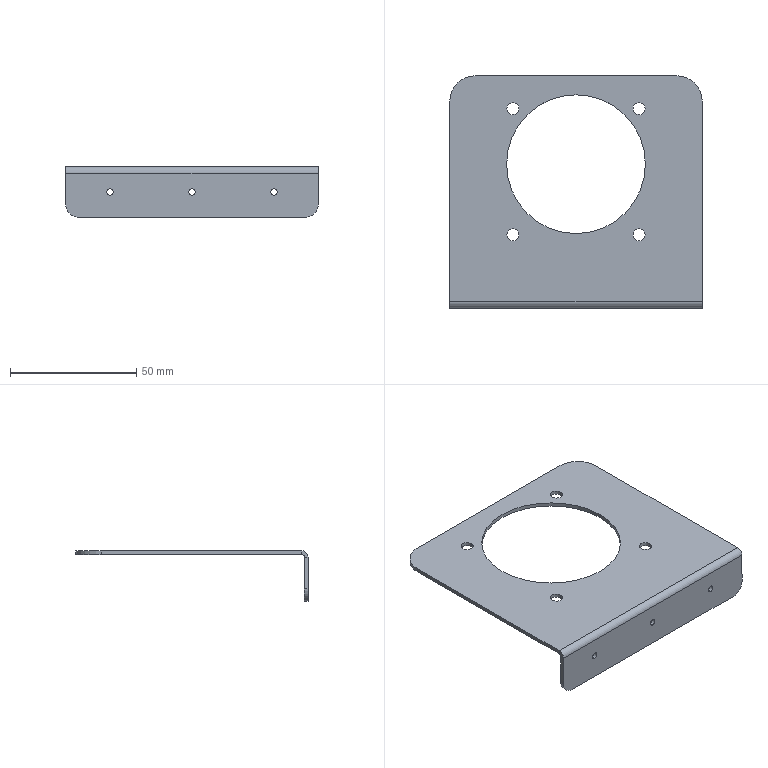Part | SolidWorks | features Fillet 2, HoleWzd 2, Cut 1, EdgeFlange 1, FlatPattern 1, ICE 1, SMBaseFlange 1, SheetMetal 1 | 1 solid | 34 faces | box 100 x 92 x 20 mm | volume 12687 mm3 | cylinder 22 | plane 12 | commonest cylinder face diameters 4.8 x8 2.5 x6 10 x2 20 x2 55 x2 2 x1
STEP:
#1=CARTESIAN_POINT('',(-32.5,-46.,-11.25));
#2=VERTEX_POINT('',#1);
#3=CARTESIAN_POINT('',(-32.5,-46.,-8.75));
#4=VERTEX_POINT('',#3);
#5=CARTESIAN_POINT('',(-32.5,-46.,-10.));
#6=DIRECTION('',(0.,1.,0.));
#7=DIRECTION('',(0.,0.,1.));
#8=AXIS2_PLACEMENT_3D('',#5,#6,#7);
#9=CIRCLE('',#8,1.25);
#10=EDGE_CURVE('',#2,#4,#9,.T.);
#11=ORIENTED_EDGE('',*,*,#10,.F.);
#12=CARTESIAN_POINT('',(-32.5,-44.5,-11.25));
#13=VERTEX_POINT('',#12);
#14=CARTESIAN_POINT('',(-32.5,-44.5,-11.25));
#15=DIRECTION('',(0.,1.,0.));
#16=VECTOR('',#15,1000.);
#17=LINE('',#14,#16);
#18=EDGE_CURVE('',#2,#13,#17,.T.);
#19=ORIENTED_EDGE('',*,*,#18,.T.);
#20=CARTESIAN_POINT('',(-32.5,-44.5,-8.75));
#21=VERTEX_POINT('',#20);
#22=CARTESIAN_POINT('',(-32.5,-44.5,-10.));
#23=DIRECTION('',(0.,1.,0.));
#24=DIRECTION('',(0.,0.,1.));
#25=AXIS2_PLACEMENT_3D('',#22,#23,#24);
#26=CIRCLE('',#25,1.25);
#27=EDGE_CURVE('',#13,#21,#26,.T.);
#28=ORIENTED_EDGE('',*,*,#27,.T.);
#29=CARTESIAN_POINT('',(-32.5,-44.5,-8.75));
#30=DIRECTION('',(0.,1.,0.));
#31=VECTOR('',#30,1000.);
#32=LINE('',#29,#31);
#33=EDGE_CURVE('',#4,#21,#32,.T.);
#34=ORIENTED_EDGE('',*,*,#33,.F.);
#35=EDGE_LOOP('',(#11,#19,#28,#34));
#36=FACE_OUTER_BOUND('',#35,.T.);
#37=CARTESIAN_POINT('',(-32.5,-44.5,-10.));
#38=DIRECTION('',(0.,1.,0.));
#39=DIRECTION('',(0.,0.,1.));
#40=AXIS2_PLACEMENT_3D('',#37,#38,#39);
#41=CYLINDRICAL_SURFACE('',#40,1.25);
#42=ADVANCED_FACE('',(#36),#41,.F.);
#43=CARTESIAN_POINT('',(0.,-46.,-11.25));
#44=VERTEX_POINT('',#43);
#45=CARTESIAN_POINT('',(0.,-46.,-8.75));
#46=VERTEX_POINT('',#45);
#47=CARTESIAN_POINT('',(0.,-46.,-10.));
#48=DIRECTION('',(0.,1.,0.));
#49=DIRECTION('',(0.,0.,1.));
#50=AXIS2_PLACEMENT_3D('',#47,#48,#49);
#51=CIRCLE('',#50,1.25);
#52=EDGE_CURVE('',#44,#46,#51,.T.);
#53=ORIENTED_EDGE('',*,*,#52,.F.);
#54=CARTESIAN_POINT('',(0.,-44.5,-11.25));
#55=VERTEX_POINT('',#54);
#56=CARTESIAN_POINT('',(0.,-44.5,-11.25));
#57=DIRECTION('',(0.,1.,0.));
#58=VECTOR('',#57,1000.);
#59=LINE('',#56,#58);
#60=EDGE_CURVE('',#44,#55,#59,.T.);
#61=ORIENTED_EDGE('',*,*,#60,.T.);
#62=CARTESIAN_POINT('',(0.,-44.5,-8.75));
#63=VERTEX_POINT('',#62);
#64=CARTESIAN_POINT('',(0.,-44.5,-10.));
#65=DIRECTION('',(0.,1.,0.));
#66=DIRECTION('',(0.,0.,1.));
#67=AXIS2_PLACEMENT_3D('',#64,#65,#66);
#68=CIRCLE('',#67,1.25);
#69=EDGE_CURVE('',#55,#63,#68,.T.);
#70=ORIENTED_EDGE('',*,*,#69,.T.);
#71=CARTESIAN_POINT('',(0.,-44.5,-8.75));
#72=DIRECTION('',(0.,1.,0.));
#73=VECTOR('',#72,1000.);
#74=LINE('',#71,#73);
#75=EDGE_CURVE('',#46,#63,#74,.T.);
#76=ORIENTED_EDGE('',*,*,#75,.F.);
#77=EDGE_LOOP('',(#53,#61,#70,#76));
#78=FACE_OUTER_BOUND('',#77,.T.);
#79=CARTESIAN_POINT('',(0.,-44.5,-10.));
#80=DIRECTION('',(0.,1.,0.));
#81=DIRECTION('',(0.,0.,1.));
#82=AXIS2_PLACEMENT_3D('',#79,#80,#81);
#83=CYLINDRICAL_SURFACE('',#82,1.25);
#84=ADVANCED_FACE('',(#78),#83,.F.);
#85=CARTESIAN_POINT('',(32.5,-46.,-11.25));
#86=VERTEX_POINT('',#85);
#87=CARTESIAN_POINT('',(32.5,-46.,-8.75));
#88=VERTEX_POINT('',#87);
#89=CARTESIAN_POINT('',(32.5,-46.,-10.));
#90=DIRECTION('',(0.,1.,0.));
#91=DIRECTION('',(0.,0.,1.));
#92=AXIS2_PLACEMENT_3D('',#89,#90,#91);
#93=CIRCLE('',#92,1.25);
#94=EDGE_CURVE('',#86,#88,#93,.T.);
#95=ORIENTED_EDGE('',*,*,#94,.F.);
#96=CARTESIAN_POINT('',(32.5,-44.5,-11.25));
#97=VERTEX_POINT('',#96);
#98=CARTESIAN_POINT('',(32.5,-44.5,-11.25));
#99=DIRECTION('',(0.,1.,0.));
#100=VECTOR('',#99,1000.);
#101=LINE('',#98,#100);
#102=EDGE_CURVE('',#86,#97,#101,.T.);
#103=ORIENTED_EDGE('',*,*,#102,.T.);
#104=CARTESIAN_POINT('',(32.5,-44.5,-8.75));
#105=VERTEX_POINT('',#104);
#106=CARTESIAN_POINT('',(32.5,-44.5,-10.));
#107=DIRECTION('',(0.,1.,0.));
#108=DIRECTION('',(0.,0.,1.));
#109=AXIS2_PLACEMENT_3D('',#106,#107,#108);
#110=CIRCLE('',#109,1.25);
#111=EDGE_CURVE('',#97,#105,#110,.T.);
#112=ORIENTED_EDGE('',*,*,#111,.T.);
#113=CARTESIAN_POINT('',(32.5,-44.5,-8.75));
#114=DIRECTION('',(0.,1.,0.));
#115=VECTOR('',#114,1000.);
#116=LINE('',#113,#115);
#117=EDGE_CURVE('',#88,#105,#116,.T.);
#118=ORIENTED_EDGE('',*,*,#117,.F.);
#119=EDGE_LOOP('',(#95,#103,#112,#118));
#120=FACE_OUTER_BOUND('',#119,.T.);
#121=CARTESIAN_POINT('',(32.5,-44.5,-10.));
#122=DIRECTION('',(0.,1.,0.));
#123=DIRECTION('',(0.,0.,1.));
#124=AXIS2_PLACEMENT_3D('',#121,#122,#123);
#125=CYLINDRICAL_SURFACE('',#124,1.25);
#126=ADVANCED_FACE('',(#120),#125,.F.);
#127=CARTESIAN_POINT('',(27.4,33.,0.));
#128=VERTEX_POINT('',#127);
#129=CARTESIAN_POINT('',(22.6,33.,0.));
#130=VERTEX_POINT('',#129);
#131=CARTESIAN_POINT('',(25.,33.,0.));
#132=DIRECTION('',(0.,0.,-1.));
#133=DIRECTION('',(-1.,0.,0.));
#134=AXIS2_PLACEMENT_3D('',#131,#132,#133);
#135=CIRCLE('',#134,2.4);
#136=EDGE_CURVE('',#128,#130,#135,.T.);
#137=ORIENTED_EDGE('',*,*,#136,.F.);
#138=CARTESIAN_POINT('',(27.4,33.,-1.5));
#139=VERTEX_POINT('',#138);
#140=CARTESIAN_POINT('',(27.4,33.,-1.5));
#141=DIRECTION('',(0.,0.,-1.));
#142=VECTOR('',#141,1000.);
#143=LINE('',#140,#142);
#144=EDGE_CURVE('',#128,#139,#143,.T.);
#145=ORIENTED_EDGE('',*,*,#144,.T.);
#146=CARTESIAN_POINT('',(22.6,33.,-1.5));
#147=VERTEX_POINT('',#146);
#148=CARTESIAN_POINT('',(25.,33.,-1.5));
#149=DIRECTION('',(0.,0.,-1.));
#150=DIRECTION('',(-1.,0.,0.));
#151=AXIS2_PLACEMENT_3D('',#148,#149,#150);
#152=CIRCLE('',#151,2.4);
#153=EDGE_CURVE('',#139,#147,#152,.T.);
#154=ORIENTED_EDGE('',*,*,#153,.T.);
#155=CARTESIAN_POINT('',(22.6,33.,-1.5));
#156=DIRECTION('',(0.,0.,-1.));
#157=VECTOR('',#156,1000.);
#158=LINE('',#155,#157);
#159=EDGE_CURVE('',#130,#147,#158,.T.);
#160=ORIENTED_EDGE('',*,*,#159,.F.);
#161=EDGE_LOOP('',(#137,#145,#154,#160));
#162=FACE_OUTER_BOUND('',#161,.T.);
#163=CARTESIAN_POINT('',(25.,33.,-1.5));
#164=DIRECTION('',(0.,0.,-1.));
#165=DIRECTION('',(-1.,0.,0.));
#166=AXIS2_PLACEMENT_3D('',#163,#164,#165);
#167=CYLINDRICAL_SURFACE('',#166,2.4);
#168=ADVANCED_FACE('',(#162),#167,.F.);
#169=CARTESIAN_POINT('',(27.4,-17.,0.));
#170=VERTEX_POINT('',#169);
#171=CARTESIAN_POINT('',(22.6,-17.,0.));
#172=VERTEX_POINT('',#171);
#173=CARTESIAN_POINT('',(25.,-17.,0.));
#174=DIRECTION('',(0.,0.,-1.));
#175=DIRECTION('',(-1.,0.,0.));
#176=AXIS2_PLACEMENT_3D('',#173,#174,#175);
#177=CIRCLE('',#176,2.4);
#178=EDGE_CURVE('',#170,#172,#177,.T.);
#179=ORIENTED_EDGE('',*,*,#178,.F.);
#180=CARTESIAN_POINT('',(27.4,-17.,-1.5));
#181=VERTEX_POINT('',#180);
#182=CARTESIAN_POINT('',(27.4,-17.,-1.5));
#183=DIRECTION('',(0.,0.,-1.));
#184=VECTOR('',#183,1000.);
#185=LINE('',#182,#184);
#186=EDGE_CURVE('',#170,#181,#185,.T.);
#187=ORIENTED_EDGE('',*,*,#186,.T.);
#188=CARTESIAN_POINT('',(22.6,-17.,-1.5));
#189=VERTEX_POINT('',#188);
#190=CARTESIAN_POINT('',(25.,-17.,-1.5));
#191=DIRECTION('',(0.,0.,-1.));
#192=DIRECTION('',(-1.,0.,0.));
#193=AXIS2_PLACEMENT_3D('',#190,#191,#192);
#194=CIRCLE('',#193,2.4);
#195=EDGE_CURVE('',#181,#189,#194,.T.);
#196=ORIENTED_EDGE('',*,*,#195,.T.);
#197=CARTESIAN_POINT('',(22.6,-17.,-1.5));
#198=DIRECTION('',(0.,0.,-1.));
#199=VECTOR('',#198,1000.);
#200=LINE('',#197,#199);
#201=EDGE_CURVE('',#172,#189,#200,.T.);
#202=ORIENTED_EDGE('',*,*,#201,.F.);
#203=EDGE_LOOP('',(#179,#187,#196,#202));
#204=FACE_OUTER_BOUND('',#203,.T.);
#205=CARTESIAN_POINT('',(25.,-17.,-1.5));
#206=DIRECTION('',(0.,0.,-1.));
#207=DIRECTION('',(-1.,0.,0.));
#208=AXIS2_PLACEMENT_3D('',#205,#206,#207);
#209=CYLINDRICAL_SURFACE('',#208,2.4);
#210=ADVANCED_FACE('',(#204),#209,.F.);
#211=CARTESIAN_POINT('',(-22.6,-17.,0.));
#212=VERTEX_POINT('',#211);
#213=CARTESIAN_POINT('',(-27.4,-17.,0.));
#214=VERTEX_POINT('',#213);
#215=CARTESIAN_POINT('',(-25.,-17.,0.));
#216=DIRECTION('',(0.,0.,-1.));
#217=DIRECTION('',(-1.,0.,0.));
#218=AXIS2_PLACEMENT_3D('',#215,#216,#217);
#219=CIRCLE('',#218,2.4);
#220=EDGE_CURVE('',#212,#214,#219,.T.);
#221=ORIENTED_EDGE('',*,*,#220,.F.);
#222=CARTESIAN_POINT('',(-22.6,-17.,-1.5));
#223=VERTEX_POINT('',#222);
#224=CARTESIAN_POINT('',(-22.6,-17.,-1.5));
#225=DIRECTION('',(0.,0.,-1.));
#226=VECTOR('',#225,1000.);
#227=LINE('',#224,#226);
#228=EDGE_CURVE('',#212,#223,#227,.T.);
#229=ORIENTED_EDGE('',*,*,#228,.T.);
#230=CARTESIAN_POINT('',(-27.4,-17.,-1.5));
#231=VERTEX_POINT('',#230);
#232=CARTESIAN_POINT('',(-25.,-17.,-1.5));
#233=DIRECTION('',(0.,0.,-1.));
#234=DIRECTION('',(-1.,0.,0.));
#235=AXIS2_PLACEMENT_3D('',#232,#233,#234);
#236=CIRCLE('',#235,2.4);
#237=EDGE_CURVE('',#223,#231,#236,.T.);
#238=ORIENTED_EDGE('',*,*,#237,.T.);
#239=CARTESIAN_POINT('',(-27.4,-17.,-1.5));
#240=DIRECTION('',(0.,0.,-1.));
#241=VECTOR('',#240,1000.);
#242=LINE('',#239,#241);
#243=EDGE_CURVE('',#214,#231,#242,.T.);
#244=ORIENTED_EDGE('',*,*,#243,.F.);
#245=EDGE_LOOP('',(#221,#229,#238,#244));
#246=FACE_OUTER_BOUND('',#245,.T.);
#247=CARTESIAN_POINT('',(-25.,-17.,-1.5));
#248=DIRECTION('',(0.,0.,-1.));
#249=DIRECTION('',(-1.,0.,0.));
#250=AXIS2_PLACEMENT_3D('',#247,#248,#249);
#251=CYLINDRICAL_SURFACE('',#250,2.4);
#252=ADVANCED_FACE('',(#246),#251,.F.);
#253=CARTESIAN_POINT('',(-22.6,33.,0.));
#254=VERTEX_POINT('',#253);
#255=CARTESIAN_POINT('',(-27.4,33.,0.));
#256=VERTEX_POINT('',#255);
#257=CARTESIAN_POINT('',(-25.,33.,0.));
#258=DIRECTION('',(0.,0.,-1.));
#259=DIRECTION('',(-1.,0.,0.));
#260=AXIS2_PLACEMENT_3D('',#257,#258,#259);
#261=CIRCLE('',#260,2.4);
#262=EDGE_CURVE('',#254,#256,#261,.T.);
#263=ORIENTED_EDGE('',*,*,#262,.F.);
#264=CARTESIAN_POINT('',(-22.6,33.,-1.5));
#265=VERTEX_POINT('',#264);
#266=CARTESIAN_POINT('',(-22.6,33.,-1.5));
#267=DIRECTION('',(0.,0.,-1.));
#268=VECTOR('',#267,1000.);
#269=LINE('',#266,#268);
#270=EDGE_CURVE('',#254,#265,#269,.T.);
#271=ORIENTED_EDGE('',*,*,#270,.T.);
#272=CARTESIAN_POINT('',(-27.4,33.,-1.5));
#273=VERTEX_POINT('',#272);
#274=CARTESIAN_POINT('',(-25.,33.,-1.5));
#275=DIRECTION('',(0.,0.,-1.));
#276=DIRECTION('',(-1.,0.,0.));
#277=AXIS2_PLACEMENT_3D('',#274,#275,#276);
#278=CIRCLE('',#277,2.4);
#279=EDGE_CURVE('',#265,#273,#278,.T.);
#280=ORIENTED_EDGE('',*,*,#279,.T.);
#281=CARTESIAN_POINT('',(-27.4,33.,-1.5));
#282=DIRECTION('',(0.,0.,-1.));
#283=VECTOR('',#282,1000.);
#284=LINE('',#281,#283);
#285=EDGE_CURVE('',#256,#273,#284,.T.);
#286=ORIENTED_EDGE('',*,*,#285,.F.);
#287=EDGE_LOOP('',(#263,#271,#280,#286));
#288=FACE_OUTER_BOUND('',#287,.T.);
#289=CARTESIAN_POINT('',(-25.,33.,-1.5));
#290=DIRECTION('',(0.,0.,-1.));
#291=DIRECTION('',(-1.,0.,0.));
#292=AXIS2_PLACEMENT_3D('',#289,#290,#291);
#293=CYLINDRICAL_SURFACE('',#292,2.4);
#294=ADVANCED_FACE('',(#288),#293,.F.);
#295=CARTESIAN_POINT('',(-27.5,11.,0.));
#296=VERTEX_POINT('',#295);
#297=CARTESIAN_POINT('',(27.5,11.,0.));
#298=VERTEX_POINT('',#297);
#299=CARTESIAN_POINT('',(0.,11.,0.));
#300=DIRECTION('',(0.,0.,1.));
#301=DIRECTION('',(1.,0.,0.));
#302=AXIS2_PLACEMENT_3D('',#299,#300,#301);
#303=CIRCLE('',#302,27.5);
#304=EDGE_CURVE('',#296,#298,#303,.T.);
#305=ORIENTED_EDGE('',*,*,#304,.T.);
#306=CARTESIAN_POINT('',(27.5,11.,-1.5));
#307=VERTEX_POINT('',#306);
#308=CARTESIAN_POINT('',(27.5,11.,8.5));
#309=DIRECTION('',(0.,0.,-1.));
#310=VECTOR('',#309,1000.);
#311=LINE('',#308,#310);
#312=EDGE_CURVE('',#298,#307,#311,.T.);
#313=ORIENTED_EDGE('',*,*,#312,.T.);
#314=CARTESIAN_POINT('',(-27.5,11.,-1.5));
#315=VERTEX_POINT('',#314);
#316=CARTESIAN_POINT('',(0.,11.,-1.5));
#317=DIRECTION('',(0.,0.,-1.));
#318=DIRECTION('',(-1.,0.,0.));
#319=AXIS2_PLACEMENT_3D('',#316,#317,#318);
#320=CIRCLE('',#319,27.5);
#321=EDGE_CURVE('',#307,#315,#320,.T.);
#322=ORIENTED_EDGE('',*,*,#321,.T.);
#323=CARTESIAN_POINT('',(-27.5,11.,8.5));
#324=DIRECTION('',(0.,0.,-1.));
#325=VECTOR('',#324,1000.);
#326=LINE('',#323,#325);
#327=EDGE_CURVE('',#296,#315,#326,.T.);
#328=ORIENTED_EDGE('',*,*,#327,.F.);
#329=EDGE_LOOP('',(#305,#313,#322,#328));
#330=FACE_OUTER_BOUND('',#329,.T.);
#331=CARTESIAN_POINT('',(0.,11.,8.5));
#332=DIRECTION('',(0.,0.,-1.));
#333=DIRECTION('',(-1.,0.,0.));
#334=AXIS2_PLACEMENT_3D('',#331,#332,#333);
#335=CYLINDRICAL_SURFACE('',#334,27.5);
#336=ADVANCED_FACE('',(#330),#335,.F.);
#337=CARTESIAN_POINT('',(0.,-44.5,-10.));
#338=DIRECTION('',(0.,1.,0.));
#339=DIRECTION('',(0.,0.,1.));
#340=AXIS2_PLACEMENT_3D('',#337,#338,#339);
#341=CIRCLE('',#340,1.25);
#342=EDGE_CURVE('',#63,#55,#341,.T.);
#343=ORIENTED_EDGE('',*,*,#342,.F.);
#344=ORIENTED_EDGE('',*,*,#69,.F.);
#345=EDGE_LOOP('',(#343,#344));
#346=FACE_BOUND('',#345,.T.);
#347=CARTESIAN_POINT('',(50.,-44.5,-2.5));
#348=VERTEX_POINT('',#347);
#349=CARTESIAN_POINT('',(50.,-44.5,-15.));
#350=VERTEX_POINT('',#349);
#351=CARTESIAN_POINT('',(50.,-44.5,0.));
#352=DIRECTION('',(0.,0.,-1.));
#353=VECTOR('',#352,1000.);
#354=LINE('',#351,#353);
#355=EDGE_CURVE('',#348,#350,#354,.T.);
#356=ORIENTED_EDGE('',*,*,#355,.T.);
#357=CARTESIAN_POINT('',(45.,-44.5,-20.));
#358=VERTEX_POINT('',#357);
#359=CARTESIAN_POINT('',(45.,-44.5,-15.));
#360=DIRECTION('',(0.,1.,0.));
#361=DIRECTION('',(0.,0.,-1.));
#362=AXIS2_PLACEMENT_3D('',#359,#360,#361);
#363=CIRCLE('',#362,5.);
#364=EDGE_CURVE('',#350,#358,#363,.T.);
#365=ORIENTED_EDGE('',*,*,#364,.T.);
#366=CARTESIAN_POINT('',(-45.,-44.5,-20.));
#367=VERTEX_POINT('',#366);
#368=CARTESIAN_POINT('',(0.,-44.5,-20.));
#369=DIRECTION('',(-1.,0.,0.));
#370=VECTOR('',#369,1000.);
#371=LINE('',#368,#370);
#372=EDGE_CURVE('',#358,#367,#371,.T.);
#373=ORIENTED_EDGE('',*,*,#372,.T.);
#374=CARTESIAN_POINT('',(-50.,-44.5,-15.));
#375=VERTEX_POINT('',#374);
#376=CARTESIAN_POINT('',(-45.,-44.5,-15.));
#377=DIRECTION('',(0.,1.,0.));
#378=DIRECTION('',(0.,0.,-1.));
#379=AXIS2_PLACEMENT_3D('',#376,#377,#378);
#380=CIRCLE('',#379,5.);
#381=EDGE_CURVE('',#367,#375,#380,.T.);
#382=ORIENTED_EDGE('',*,*,#381,.T.);
#383=CARTESIAN_POINT('',(-50.,-44.5,-2.5));
#384=VERTEX_POINT('',#383);
#385=CARTESIAN_POINT('',(-50.,-44.5,0.));
#386=DIRECTION('',(0.,0.,1.));
#387=VECTOR('',#386,1000.);
#388=LINE('',#385,#387);
#389=EDGE_CURVE('',#375,#384,#388,.T.);
#390=ORIENTED_EDGE('',*,*,#389,.T.);
#391=CARTESIAN_POINT('',(50.,-44.5,-2.5));
#392=DIRECTION('',(-1.,0.,0.));
#393=VECTOR('',#392,1000.);
#394=LINE('',#391,#393);
#395=EDGE_CURVE('',#348,#384,#394,.T.);
#396=ORIENTED_EDGE('',*,*,#395,.F.);
#397=EDGE_LOOP('',(#356,#365,#373,#382,#390,#396));
#398=FACE_OUTER_BOUND('',#397,.T.);
#399=CARTESIAN_POINT('',(32.5,-44.5,-10.));
#400=DIRECTION('',(0.,1.,0.));
#401=DIRECTION('',(0.,0.,1.));
#402=AXIS2_PLACEMENT_3D('',#399,#400,#401);
#403=CIRCLE('',#402,1.25);
#404=EDGE_CURVE('',#105,#97,#403,.T.);
#405=ORIENTED_EDGE('',*,*,#404,.F.);
#406=ORIENTED_EDGE('',*,*,#111,.F.);
#407=EDGE_LOOP('',(#405,#406));
#408=FACE_BOUND('',#407,.T.);
#409=CARTESIAN_POINT('',(-32.5,-44.5,-10.));
#410=DIRECTION('',(0.,1.,0.));
#411=DIRECTION('',(0.,0.,1.));
#412=AXIS2_PLACEMENT_3D('',#409,#410,#411);
#413=CIRCLE('',#412,1.25);
#414=EDGE_CURVE('',#21,#13,#413,.T.);
#415=ORIENTED_EDGE('',*,*,#414,.F.);
#416=ORIENTED_EDGE('',*,*,#27,.F.);
#417=EDGE_LOOP('',(#415,#416));
#418=FACE_BOUND('',#417,.T.);
#419=CARTESIAN_POINT('',(0.,-44.5,0.));
#420=DIRECTION('',(0.,-1.,0.));
#421=DIRECTION('',(0.,0.,-1.));
#422=AXIS2_PLACEMENT_3D('',#419,#420,#421);
#423=PLANE('',#422);
#424=ADVANCED_FACE('',(#346,#398,#408,#418),#423,.F.);
#425=CARTESIAN_POINT('',(-32.5,-46.,-10.));
#426=DIRECTION('',(0.,1.,0.));
#427=DIRECTION('',(0.,0.,1.));
#428=AXIS2_PLACEMENT_3D('',#425,#426,#427);
#429=CIRCLE('',#428,1.25);
#430=EDGE_CURVE('',#4,#2,#429,.T.);
#431=ORIENTED_EDGE('',*,*,#430,.T.);
#432=ORIENTED_EDGE('',*,*,#10,.T.);
#433=EDGE_LOOP('',(#431,#432));
#434=FACE_BOUND('',#433,.T.);
#435=CARTESIAN_POINT('',(0.,-46.,-10.));
#436=DIRECTION('',(0.,1.,0.));
#437=DIRECTION('',(0.,0.,1.));
#438=AXIS2_PLACEMENT_3D('',#435,#436,#437);
#439=CIRCLE('',#438,1.25);
#440=EDGE_CURVE('',#46,#44,#439,.T.);
#441=ORIENTED_EDGE('',*,*,#440,.T.);
#442=ORIENTED_EDGE('',*,*,#52,.T.);
#443=EDGE_LOOP('',(#441,#442));
#444=FACE_BOUND('',#443,.T.);
#445=CARTESIAN_POINT('',(45.,-46.,-20.));
#446=VERTEX_POINT('',#445);
#447=CARTESIAN_POINT('',(-45.,-46.,-20.));
#448=VERTEX_POINT('',#447);
#449=CARTESIAN_POINT('',(-50.,-46.,-20.));
#450=DIRECTION('',(-1.,0.,0.));
#451=VECTOR('',#450,1000.);
#452=LINE('',#449,#451);
#453=EDGE_CURVE('',#446,#448,#452,.T.);
#454=ORIENTED_EDGE('',*,*,#453,.F.);
#455=CARTESIAN_POINT('',(50.,-46.,-15.));
#456=VERTEX_POINT('',#455);
#457=CARTESIAN_POINT('',(45.,-46.,-15.));
#458=DIRECTION('',(0.,-1.,0.));
#459=DIRECTION('',(0.,0.,-1.));
#460=AXIS2_PLACEMENT_3D('',#457,#458,#459);
#461=CIRCLE('',#460,5.);
#462=EDGE_CURVE('',#446,#456,#461,.T.);
#463=ORIENTED_EDGE('',*,*,#462,.T.);
#464=CARTESIAN_POINT('',(50.,-46.,-2.5));
#465=VERTEX_POINT('',#464);
#466=CARTESIAN_POINT('',(50.,-46.,-20.));
#467=DIRECTION('',(0.,0.,-1.));
#468=VECTOR('',#467,1000.);
#469=LINE('',#466,#468);
#470=EDGE_CURVE('',#465,#456,#469,.T.);
#471=ORIENTED_EDGE('',*,*,#470,.F.);
#472=CARTESIAN_POINT('',(-50.,-46.,-2.5));
#473=VERTEX_POINT('',#472);
#474=CARTESIAN_POINT('',(0.,-46.,-2.5));
#475=DIRECTION('',(-1.,0.,0.));
#476=VECTOR('',#475,1000.);
#477=LINE('',#474,#476);
#478=EDGE_CURVE('',#465,#473,#477,.T.);
#479=ORIENTED_EDGE('',*,*,#478,.T.);
#480=CARTESIAN_POINT('',(-50.,-46.,-15.));
#481=VERTEX_POINT('',#480);
#482=CARTESIAN_POINT('',(-50.,-46.,-1.5));
#483=DIRECTION('',(0.,0.,1.));
#484=VECTOR('',#483,1000.);
#485=LINE('',#482,#484);
#486=EDGE_CURVE('',#481,#473,#485,.T.);
#487=ORIENTED_EDGE('',*,*,#486,.F.);
#488=CARTESIAN_POINT('',(-45.,-46.,-15.));
#489=DIRECTION('',(0.,-1.,0.));
#490=DIRECTION('',(0.,0.,-1.));
#491=AXIS2_PLACEMENT_3D('',#488,#489,#490);
#492=CIRCLE('',#491,5.);
#493=EDGE_CURVE('',#481,#448,#492,.T.);
#494=ORIENTED_EDGE('',*,*,#493,.T.);
#495=EDGE_LOOP('',(#454,#463,#471,#479,#487,#494));
#496=FACE_OUTER_BOUND('',#495,.T.);
#497=CARTESIAN_POINT('',(32.5,-46.,-10.));
#498=DIRECTION('',(0.,1.,0.));
#499=DIRECTION('',(0.,0.,1.));
#500=AXIS2_PLACEMENT_3D('',#497,#498,#499);
#501=CIRCLE('',#500,1.25);
#502=EDGE_CURVE('',#88,#86,#501,.T.);
#503=ORIENTED_EDGE('',*,*,#502,.T.);
#504=ORIENTED_EDGE('',*,*,#94,.T.);
#505=EDGE_LOOP('',(#503,#504));
#506=FACE_BOUND('',#505,.T.);
#507=CARTESIAN_POINT('',(0.,-46.,0.));
#508=DIRECTION('',(0.,-1.,0.));
#509=DIRECTION('',(0.,0.,-1.));
#510=AXIS2_PLACEMENT_3D('',#507,#508,#509);
#511=PLANE('',#510);
#512=ADVANCED_FACE('',(#434,#444,#496,#506),#511,.T.);
#513=CARTESIAN_POINT('',(25.,33.,-1.5));
#514=DIRECTION('',(0.,0.,-1.));
#515=DIRECTION('',(-1.,0.,0.));
#516=AXIS2_PLACEMENT_3D('',#513,#514,#515);
#517=CIRCLE('',#516,2.4);
#518=EDGE_CURVE('',#147,#139,#517,.T.);
#519=ORIENTED_EDGE('',*,*,#518,.F.);
#520=ORIENTED_EDGE('',*,*,#153,.F.);
#521=EDGE_LOOP('',(#519,#520));
#522=FACE_BOUND('',#521,.T.);
#523=CARTESIAN_POINT('',(25.,-17.,-1.5));
#524=DIRECTION('',(0.,0.,-1.));
#525=DIRECTION('',(-1.,0.,0.));
#526=AXIS2_PLACEMENT_3D('',#523,#524,#525);
#527=CIRCLE('',#526,2.4);
#528=EDGE_CURVE('',#189,#181,#527,.T.);
#529=ORIENTED_EDGE('',*,*,#528,.F.);
#530=ORIENTED_EDGE('',*,*,#195,.F.);
#531=EDGE_LOOP('',(#529,#530));
#532=FACE_BOUND('',#531,.T.);
#533=CARTESIAN_POINT('',(-25.,-17.,-1.5));
#534=DIRECTION('',(0.,0.,-1.));
#535=DIRECTION('',(-1.,0.,0.));
#536=AXIS2_PLACEMENT_3D('',#533,#534,#535);
#537=CIRCLE('',#536,2.4);
#538=EDGE_CURVE('',#231,#223,#537,.T.);
#539=ORIENTED_EDGE('',*,*,#538,.F.);
#540=ORIENTED_EDGE('',*,*,#237,.F.);
#541=EDGE_LOOP('',(#539,#540));
#542=FACE_BOUND('',#541,.T.);
#543=CARTESIAN_POINT('',(0.,11.,-1.5));
#544=DIRECTION('',(0.,0.,-1.));
#545=DIRECTION('',(-1.,0.,0.));
#546=AXIS2_PLACEMENT_3D('',#543,#544,#545);
#547=CIRCLE('',#546,27.5);
#548=EDGE_CURVE('',#315,#307,#547,.T.);
#549=ORIENTED_EDGE('',*,*,#548,.F.);
#550=ORIENTED_EDGE('',*,*,#321,.F.);
#551=EDGE_LOOP('',(#549,#550));
#552=FACE_BOUND('',#551,.T.);
#553=CARTESIAN_POINT('',(40.,46.,-1.5));
#554=VERTEX_POINT('',#553);
#555=CARTESIAN_POINT('',(-40.,46.,-1.5));
#556=VERTEX_POINT('',#555);
#557=CARTESIAN_POINT('',(-50.,46.,-1.5));
#558=DIRECTION('',(-1.,0.,0.));
#559=VECTOR('',#558,1000.);
#560=LINE('',#557,#559);
#561=EDGE_CURVE('',#554,#556,#560,.T.);
#562=ORIENTED_EDGE('',*,*,#561,.F.);
#563=CARTESIAN_POINT('',(50.,36.,-1.5));
#564=VERTEX_POINT('',#563);
#565=CARTESIAN_POINT('',(40.,36.,-1.5));
#566=DIRECTION('',(0.,0.,-1.));
#567=DIRECTION('',(1.,0.,0.));
#568=AXIS2_PLACEMENT_3D('',#565,#566,#567);
#569=CIRCLE('',#568,10.);
#570=EDGE_CURVE('',#554,#564,#569,.T.);
#571=ORIENTED_EDGE('',*,*,#570,.T.);
#572=CARTESIAN_POINT('',(50.,-43.5,-1.5));
#573=VERTEX_POINT('',#572);
#574=CARTESIAN_POINT('',(50.,46.,-1.5));
#575=DIRECTION('',(0.,1.,0.));
#576=VECTOR('',#575,1000.);
#577=LINE('',#574,#576);
#578=EDGE_CURVE('',#573,#564,#577,.T.);
#579=ORIENTED_EDGE('',*,*,#578,.F.);
#580=CARTESIAN_POINT('',(-50.,-43.5,-1.5));
#581=VERTEX_POINT('',#580);
#582=CARTESIAN_POINT('',(-50.,-43.5,-1.5));
#583=DIRECTION('',(1.,0.,0.));
#584=VECTOR('',#583,1000.);
#585=LINE('',#582,#584);
#586=EDGE_CURVE('',#581,#573,#585,.T.);
#587=ORIENTED_EDGE('',*,*,#586,.F.);
#588=CARTESIAN_POINT('',(-50.,36.,-1.5));
#589=VERTEX_POINT('',#588);
#590=CARTESIAN_POINT('',(-50.,46.,-1.5));
#591=DIRECTION('',(0.,-1.,0.));
#592=VECTOR('',#591,1000.);
#593=LINE('',#590,#592);
#594=EDGE_CURVE('',#589,#581,#593,.T.);
#595=ORIENTED_EDGE('',*,*,#594,.F.);
#596=CARTESIAN_POINT('',(-40.,36.,-1.5));
#597=DIRECTION('',(0.,0.,-1.));
#598=DIRECTION('',(1.,0.,0.));
#599=AXIS2_PLACEMENT_3D('',#596,#597,#598);
#600=CIRCLE('',#599,10.);
#601=EDGE_CURVE('',#589,#556,#600,.T.);
#602=ORIENTED_EDGE('',*,*,#601,.T.);
#603=EDGE_LOOP('',(#562,#571,#579,#587,#595,#602));
#604=FACE_OUTER_BOUND('',#603,.T.);
#605=CARTESIAN_POINT('',(-25.,33.,-1.5));
#606=DIRECTION('',(0.,0.,-1.));
#607=DIRECTION('',(-1.,0.,0.));
#608=AXIS2_PLACEMENT_3D('',#605,#606,#607);
#609=CIRCLE('',#608,2.4);
#610=EDGE_CURVE('',#273,#265,#609,.T.);
#611=ORIENTED_EDGE('',*,*,#610,.F.);
#612=ORIENTED_EDGE('',*,*,#279,.F.);
#613=EDGE_LOOP('',(#611,#612));
#614=FACE_BOUND('',#613,.T.);
#615=CARTESIAN_POINT('',(0.,0.,-1.5));
#616=DIRECTION('',(0.,0.,1.));
#617=DIRECTION('',(1.,0.,0.));
#618=AXIS2_PLACEMENT_3D('',#615,#616,#617);
#619=PLANE('',#618);
#620=ADVANCED_FACE('',(#522,#532,#542,#552,#604,#614),#619,.F.);
#621=CARTESIAN_POINT('',(25.,33.,0.));
#622=DIRECTION('',(0.,0.,-1.));
#623=DIRECTION('',(-1.,0.,0.));
#624=AXIS2_PLACEMENT_3D('',#621,#622,#623);
#625=CIRCLE('',#624,2.4);
#626=EDGE_CURVE('',#130,#128,#625,.T.);
#627=ORIENTED_EDGE('',*,*,#626,.T.);
#628=ORIENTED_EDGE('',*,*,#136,.T.);
#629=EDGE_LOOP('',(#627,#628));
#630=FACE_BOUND('',#629,.T.);
#631=CARTESIAN_POINT('',(25.,-17.,0.));
#632=DIRECTION('',(0.,0.,-1.));
#633=DIRECTION('',(-1.,0.,0.));
#634=AXIS2_PLACEMENT_3D('',#631,#632,#633);
#635=CIRCLE('',#634,2.4);
#636=EDGE_CURVE('',#172,#170,#635,.T.);
#637=ORIENTED_EDGE('',*,*,#636,.T.);
#638=ORIENTED_EDGE('',*,*,#178,.T.);
#639=EDGE_LOOP('',(#637,#638));
#640=FACE_BOUND('',#639,.T.);
#641=CARTESIAN_POINT('',(-25.,-17.,0.));
#642=DIRECTION('',(0.,0.,-1.));
#643=DIRECTION('',(-1.,0.,0.));
#644=AXIS2_PLACEMENT_3D('',#641,#642,#643);
#645=CIRCLE('',#644,2.4);
#646=EDGE_CURVE('',#214,#212,#645,.T.);
#647=ORIENTED_EDGE('',*,*,#646,.T.);
#648=ORIENTED_EDGE('',*,*,#220,.T.);
#649=EDGE_LOOP('',(#647,#648));
#650=FACE_BOUND('',#649,.T.);
#651=CARTESIAN_POINT('',(50.,-43.5,0.));
#652=VERTEX_POINT('',#651);
#653=CARTESIAN_POINT('',(50.,36.,0.));
#654=VERTEX_POINT('',#653);
#655=CARTESIAN_POINT('',(50.,46.,0.));
#656=DIRECTION('',(0.,1.,0.));
#657=VECTOR('',#656,1000.);
#658=LINE('',#655,#657);
#659=EDGE_CURVE('',#652,#654,#658,.T.);
#660=ORIENTED_EDGE('',*,*,#659,.T.);
#661=CARTESIAN_POINT('',(40.,46.,0.));
#662=VERTEX_POINT('',#661);
#663=CARTESIAN_POINT('',(40.,36.,0.));
#664=DIRECTION('',(0.,0.,1.));
#665=DIRECTION('',(1.,0.,0.));
#666=AXIS2_PLACEMENT_3D('',#663,#664,#665);
#667=CIRCLE('',#666,10.);
#668=EDGE_CURVE('',#654,#662,#667,.T.);
#669=ORIENTED_EDGE('',*,*,#668,.T.);
#670=CARTESIAN_POINT('',(-40.,46.,0.));
#671=VERTEX_POINT('',#670);
#672=CARTESIAN_POINT('',(-50.,46.,0.));
#673=DIRECTION('',(-1.,0.,0.));
#674=VECTOR('',#673,1000.);
#675=LINE('',#672,#674);
#676=EDGE_CURVE('',#662,#671,#675,.T.);
#677=ORIENTED_EDGE('',*,*,#676,.T.);
#678=CARTESIAN_POINT('',(-50.,36.,0.));
#679=VERTEX_POINT('',#678);
#680=CARTESIAN_POINT('',(-40.,36.,0.));
#681=DIRECTION('',(0.,0.,1.));
#682=DIRECTION('',(1.,0.,0.));
#683=AXIS2_PLACEMENT_3D('',#680,#681,#682);
#684=CIRCLE('',#683,10.);
#685=EDGE_CURVE('',#671,#679,#684,.T.);
#686=ORIENTED_EDGE('',*,*,#685,.T.);
#687=CARTESIAN_POINT('',(-50.,-43.5,0.));
#688=VERTEX_POINT('',#687);
#689=CARTESIAN_POINT('',(-50.,46.,0.));
#690=DIRECTION('',(0.,-1.,0.));
#691=VECTOR('',#690,1000.);
#692=LINE('',#689,#691);
#693=EDGE_CURVE('',#679,#688,#692,.T.);
#694=ORIENTED_EDGE('',*,*,#693,.T.);
#695=CARTESIAN_POINT('',(-50.,-43.5,0.));
#696=DIRECTION('',(1.,0.,0.));
#697=VECTOR('',#696,1000.);
#698=LINE('',#695,#697);
#699=EDGE_CURVE('',#688,#652,#698,.T.);
#700=ORIENTED_EDGE('',*,*,#699,.T.);
#701=EDGE_LOOP('',(#660,#669,#677,#686,#694,#700));
#702=FACE_OUTER_BOUND('',#701,.T.);
#703=ORIENTED_EDGE('',*,*,#304,.F.);
#704=CARTESIAN_POINT('',(0.,11.,0.));
#705=DIRECTION('',(0.,0.,1.));
#706=DIRECTION('',(1.,0.,0.));
#707=AXIS2_PLACEMENT_3D('',#704,#705,#706);
#708=CIRCLE('',#707,27.5);
#709=EDGE_CURVE('',#298,#296,#708,.T.);
#710=ORIENTED_EDGE('',*,*,#709,.F.);
#711=EDGE_LOOP('',(#703,#710));
#712=FACE_BOUND('',#711,.T.);
#713=CARTESIAN_POINT('',(-25.,33.,0.));
#714=DIRECTION('',(0.,0.,-1.));
#715=DIRECTION('',(-1.,0.,0.));
#716=AXIS2_PLACEMENT_3D('',#713,#714,#715);
#717=CIRCLE('',#716,2.4);
#718=EDGE_CURVE('',#256,#254,#717,.T.);
#719=ORIENTED_EDGE('',*,*,#718,.T.);
#720=ORIENTED_EDGE('',*,*,#262,.T.);
#721=EDGE_LOOP('',(#719,#720));
#722=FACE_BOUND('',#721,.T.);
#723=CARTESIAN_POINT('',(0.,0.,0.));
#724=DIRECTION('',(0.,0.,1.));
#725=DIRECTION('',(1.,0.,0.));
#726=AXIS2_PLACEMENT_3D('',#723,#724,#725);
#727=PLANE('',#726);
#728=ADVANCED_FACE('',(#630,#640,#650,#702,#712,#722),#727,.T.);
#729=ORIENTED_EDGE('',*,*,#693,.F.);
#730=CARTESIAN_POINT('',(-50.,36.,-1.5));
#731=DIRECTION('',(0.,0.,-1.));
#732=VECTOR('',#731,1000.);
#733=LINE('',#730,#732);
#734=EDGE_CURVE('',#679,#589,#733,.T.);
#735=ORIENTED_EDGE('',*,*,#734,.T.);
#736=ORIENTED_EDGE('',*,*,#594,.T.);
#737=CARTESIAN_POINT('',(-50.,-43.5,-1.5));
#738=DIRECTION('',(0.,0.,1.));
#739=VECTOR('',#738,1000.);
#740=LINE('',#737,#739);
#741=EDGE_CURVE('',#581,#688,#740,.T.);
#742=ORIENTED_EDGE('',*,*,#741,.T.);
#743=EDGE_LOOP('',(#729,#735,#736,#742));
#744=FACE_OUTER_BOUND('',#743,.T.);
#745=CARTESIAN_POINT('',(-50.,46.,-1.5));
#746=DIRECTION('',(-1.,0.,0.));
#747=DIRECTION('',(0.,-1.,0.));
#748=AXIS2_PLACEMENT_3D('',#745,#746,#747);
#749=PLANE('',#748);
#750=ADVANCED_FACE('',(#744),#749,.T.);
#751=ORIENTED_EDGE('',*,*,#578,.T.);
#752=CARTESIAN_POINT('',(50.,36.,-1.5));
#753=DIRECTION('',(0.,0.,1.));
#754=VECTOR('',#753,1000.);
#755=LINE('',#752,#754);
#756=EDGE_CURVE('',#564,#654,#755,.T.);
#757=ORIENTED_EDGE('',*,*,#756,.T.);
#758=ORIENTED_EDGE('',*,*,#659,.F.);
#759=CARTESIAN_POINT('',(50.,-43.5,-1.5));
#760=DIRECTION('',(0.,0.,1.));
#761=VECTOR('',#760,1000.);
#762=LINE('',#759,#761);
#763=EDGE_CURVE('',#573,#652,#762,.T.);
#764=ORIENTED_EDGE('',*,*,#763,.F.);
#765=EDGE_LOOP('',(#751,#757,#758,#764));
#766=FACE_OUTER_BOUND('',#765,.T.);
#767=CARTESIAN_POINT('',(50.,46.,-1.5));
#768=DIRECTION('',(1.,0.,0.));
#769=DIRECTION('',(0.,1.,0.));
#770=AXIS2_PLACEMENT_3D('',#767,#768,#769);
#771=PLANE('',#770);
#772=ADVANCED_FACE('',(#766),#771,.T.);
#773=ORIENTED_EDGE('',*,*,#676,.F.);
#774=CARTESIAN_POINT('',(40.,46.,-1.5));
#775=DIRECTION('',(0.,0.,-1.));
#776=VECTOR('',#775,1000.);
#777=LINE('',#774,#776);
#778=EDGE_CURVE('',#662,#554,#777,.T.);
#779=ORIENTED_EDGE('',*,*,#778,.T.);
#780=ORIENTED_EDGE('',*,*,#561,.T.);
#781=CARTESIAN_POINT('',(-40.,46.,-1.5));
#782=DIRECTION('',(0.,0.,1.));
#783=VECTOR('',#782,1000.);
#784=LINE('',#781,#783);
#785=EDGE_CURVE('',#556,#671,#784,.T.);
#786=ORIENTED_EDGE('',*,*,#785,.T.);
#787=EDGE_LOOP('',(#773,#779,#780,#786));
#788=FACE_OUTER_BOUND('',#787,.T.);
#789=CARTESIAN_POINT('',(-50.,46.,-1.5));
#790=DIRECTION('',(0.,1.,0.));
#791=DIRECTION('',(0.,0.,1.));
#792=AXIS2_PLACEMENT_3D('',#789,#790,#791);
#793=PLANE('',#792);
#794=ADVANCED_FACE('',(#788),#793,.T.);
#795=CARTESIAN_POINT('',(50.,-46.,-2.5));
#796=DIRECTION('',(0.,-1.,0.));
#797=VECTOR('',#796,1000.);
#798=LINE('',#795,#797);
#799=EDGE_CURVE('',#348,#465,#798,.T.);
#800=ORIENTED_EDGE('',*,*,#799,.F.);
#801=CARTESIAN_POINT('',(50.,-43.5,-2.5));
#802=DIRECTION('',(1.,0.,0.));
#803=DIRECTION('',(0.,0.,1.));
#804=AXIS2_PLACEMENT_3D('',#801,#802,#803);
#805=CIRCLE('',#804,1.);
#806=EDGE_CURVE('',#573,#348,#805,.T.);
#807=ORIENTED_EDGE('',*,*,#806,.F.);
#808=ORIENTED_EDGE('',*,*,#763,.T.);
#809=CARTESIAN_POINT('',(50.,-43.5,-2.5));
#810=DIRECTION('',(1.,0.,0.));
#811=DIRECTION('',(0.,0.,1.));
#812=AXIS2_PLACEMENT_3D('',#809,#810,#811);
#813=CIRCLE('',#812,2.5);
#814=EDGE_CURVE('',#652,#465,#813,.T.);
#815=ORIENTED_EDGE('',*,*,#814,.T.);
#816=EDGE_LOOP('',(#800,#807,#808,#815));
#817=FACE_OUTER_BOUND('',#816,.T.);
#818=CARTESIAN_POINT('',(50.,-43.5,-2.5));
#819=DIRECTION('',(1.,0.,0.));
#820=DIRECTION('',(0.,0.,-1.));
#821=AXIS2_PLACEMENT_3D('',#818,#819,#820);
#822=PLANE('',#821);
#823=ADVANCED_FACE('',(#817),#822,.T.);
#824=CARTESIAN_POINT('',(-50.,-43.5,-2.5));
#825=DIRECTION('',(-1.,0.,0.));
#826=DIRECTION('',(0.,0.,1.));
#827=AXIS2_PLACEMENT_3D('',#824,#825,#826);
#828=CIRCLE('',#827,1.);
#829=EDGE_CURVE('',#384,#581,#828,.T.);
#830=ORIENTED_EDGE('',*,*,#829,.F.);
#831=CARTESIAN_POINT('',(-50.,-44.5,-2.5));
#832=DIRECTION('',(0.,-1.,0.));
#833=VECTOR('',#832,1000.);
#834=LINE('',#831,#833);
#835=EDGE_CURVE('',#384,#473,#834,.T.);
#836=ORIENTED_EDGE('',*,*,#835,.T.);
#837=CARTESIAN_POINT('',(-50.,-43.5,-2.5));
#838=DIRECTION('',(-1.,0.,0.));
#839=DIRECTION('',(0.,0.,1.));
#840=AXIS2_PLACEMENT_3D('',#837,#838,#839);
#841=CIRCLE('',#840,2.5);
#842=EDGE_CURVE('',#473,#688,#841,.T.);
#843=ORIENTED_EDGE('',*,*,#842,.T.);
#844=ORIENTED_EDGE('',*,*,#741,.F.);
#845=EDGE_LOOP('',(#830,#836,#843,#844));
#846=FACE_OUTER_BOUND('',#845,.T.);
#847=CARTESIAN_POINT('',(-50.,-43.5,-2.5));
#848=DIRECTION('',(1.,0.,0.));
#849=DIRECTION('',(0.,0.,-1.));
#850=AXIS2_PLACEMENT_3D('',#847,#848,#849);
#851=PLANE('',#850);
#852=ADVANCED_FACE('',(#846),#851,.F.);
#853=ORIENTED_EDGE('',*,*,#699,.F.);
#854=ORIENTED_EDGE('',*,*,#842,.F.);
#855=ORIENTED_EDGE('',*,*,#478,.F.);
#856=ORIENTED_EDGE('',*,*,#814,.F.);
#857=EDGE_LOOP('',(#853,#854,#855,#856));
#858=FACE_OUTER_BOUND('',#857,.T.);
#859=CARTESIAN_POINT('',(-50.,-43.5,-2.5));
#860=DIRECTION('',(-1.,0.,0.));
#861=DIRECTION('',(0.,-1.,0.));
#862=AXIS2_PLACEMENT_3D('',#859,#860,#861);
#863=CYLINDRICAL_SURFACE('',#862,2.5);
#864=ADVANCED_FACE('',(#858),#863,.T.);
#865=ORIENTED_EDGE('',*,*,#586,.T.);
#866=ORIENTED_EDGE('',*,*,#806,.T.);
#867=ORIENTED_EDGE('',*,*,#395,.T.);
#868=ORIENTED_EDGE('',*,*,#829,.T.);
#869=EDGE_LOOP('',(#865,#866,#867,#868));
#870=FACE_OUTER_BOUND('',#869,.T.);
#871=CARTESIAN_POINT('',(-50.,-43.5,-2.5));
#872=DIRECTION('',(-1.,0.,0.));
#873=DIRECTION('',(0.,-1.,0.));
#874=AXIS2_PLACEMENT_3D('',#871,#872,#873);
#875=CYLINDRICAL_SURFACE('',#874,1.);
#876=ADVANCED_FACE('',(#870),#875,.F.);
#877=ORIENTED_EDGE('',*,*,#389,.F.);
#878=CARTESIAN_POINT('',(-50.,-46.,-15.));
#879=DIRECTION('',(0.,-1.,0.));
#880=VECTOR('',#879,1000.);
#881=LINE('',#878,#880);
#882=EDGE_CURVE('',#375,#481,#881,.T.);
#883=ORIENTED_EDGE('',*,*,#882,.T.);
#884=ORIENTED_EDGE('',*,*,#486,.T.);
#885=ORIENTED_EDGE('',*,*,#835,.F.);
#886=EDGE_LOOP('',(#877,#883,#884,#885));
#887=FACE_OUTER_BOUND('',#886,.T.);
#888=CARTESIAN_POINT('',(-50.,-46.,-1.5));
#889=DIRECTION('',(-1.,0.,0.));
#890=DIRECTION('',(0.,0.,1.));
#891=AXIS2_PLACEMENT_3D('',#888,#889,#890);
#892=PLANE('',#891);
#893=ADVANCED_FACE('',(#887),#892,.T.);
#894=ORIENTED_EDGE('',*,*,#470,.T.);
#895=CARTESIAN_POINT('',(50.,-46.,-15.));
#896=DIRECTION('',(0.,1.,0.));
#897=VECTOR('',#896,1000.);
#898=LINE('',#895,#897);
#899=EDGE_CURVE('',#456,#350,#898,.T.);
#900=ORIENTED_EDGE('',*,*,#899,.T.);
#901=ORIENTED_EDGE('',*,*,#355,.F.);
#902=ORIENTED_EDGE('',*,*,#799,.T.);
#903=EDGE_LOOP('',(#894,#900,#901,#902));
#904=FACE_OUTER_BOUND('',#903,.T.);
#905=CARTESIAN_POINT('',(50.,-46.,-20.));
#906=DIRECTION('',(1.,0.,0.));
#907=DIRECTION('',(0.,0.,-1.));
#908=AXIS2_PLACEMENT_3D('',#905,#906,#907);
#909=PLANE('',#908);
#910=ADVANCED_FACE('',(#904),#909,.T.);
#911=ORIENTED_EDGE('',*,*,#372,.F.);
#912=CARTESIAN_POINT('',(45.,-46.,-20.));
#913=DIRECTION('',(0.,-1.,0.));
#914=VECTOR('',#913,1000.);
#915=LINE('',#912,#914);
#916=EDGE_CURVE('',#358,#446,#915,.T.);
#917=ORIENTED_EDGE('',*,*,#916,.T.);
#918=ORIENTED_EDGE('',*,*,#453,.T.);
#919=CARTESIAN_POINT('',(-45.,-46.,-20.));
#920=DIRECTION('',(0.,1.,0.));
#921=VECTOR('',#920,1000.);
#922=LINE('',#919,#921);
#923=EDGE_CURVE('',#448,#367,#922,.T.);
#924=ORIENTED_EDGE('',*,*,#923,.T.);
#925=EDGE_LOOP('',(#911,#917,#918,#924));
#926=FACE_OUTER_BOUND('',#925,.T.);
#927=CARTESIAN_POINT('',(-50.,-46.,-20.));
#928=DIRECTION('',(0.,0.,-1.));
#929=DIRECTION('',(0.,1.,0.));
#930=AXIS2_PLACEMENT_3D('',#927,#928,#929);
#931=PLANE('',#930);
#932=ADVANCED_FACE('',(#926),#931,.T.);
#933=ORIENTED_EDGE('',*,*,#570,.F.);
#934=ORIENTED_EDGE('',*,*,#778,.F.);
#935=ORIENTED_EDGE('',*,*,#668,.F.);
#936=ORIENTED_EDGE('',*,*,#756,.F.);
#937=EDGE_LOOP('',(#933,#934,#935,#936));
#938=FACE_OUTER_BOUND('',#937,.T.);
#939=CARTESIAN_POINT('',(40.,36.,-1.5));
#940=DIRECTION('',(0.,0.,1.));
#941=DIRECTION('',(1.,0.,0.));
#942=AXIS2_PLACEMENT_3D('',#939,#940,#941);
#943=CYLINDRICAL_SURFACE('',#942,10.);
#944=ADVANCED_FACE('',(#938),#943,.T.);
#945=ORIENTED_EDGE('',*,*,#601,.F.);
#946=ORIENTED_EDGE('',*,*,#734,.F.);
#947=ORIENTED_EDGE('',*,*,#685,.F.);
#948=ORIENTED_EDGE('',*,*,#785,.F.);
#949=EDGE_LOOP('',(#945,#946,#947,#948));
#950=FACE_OUTER_BOUND('',#949,.T.);
#951=CARTESIAN_POINT('',(-40.,36.,-1.5));
#952=DIRECTION('',(0.,0.,1.));
#953=DIRECTION('',(1.,0.,0.));
#954=AXIS2_PLACEMENT_3D('',#951,#952,#953);
#955=CYLINDRICAL_SURFACE('',#954,10.);
#956=ADVANCED_FACE('',(#950),#955,.T.);
#957=ORIENTED_EDGE('',*,*,#312,.F.);
#958=ORIENTED_EDGE('',*,*,#709,.T.);
#959=ORIENTED_EDGE('',*,*,#327,.T.);
#960=ORIENTED_EDGE('',*,*,#548,.T.);
#961=EDGE_LOOP('',(#957,#958,#959,#960));
#962=FACE_OUTER_BOUND('',#961,.T.);
#963=CARTESIAN_POINT('',(0.,11.,8.5));
#964=DIRECTION('',(0.,0.,-1.));
#965=DIRECTION('',(-1.,0.,0.));
#966=AXIS2_PLACEMENT_3D('',#963,#964,#965);
#967=CYLINDRICAL_SURFACE('',#966,27.5);
#968=ADVANCED_FACE('',(#962),#967,.F.);
#969=ORIENTED_EDGE('',*,*,#270,.F.);
#970=ORIENTED_EDGE('',*,*,#718,.F.);
#971=ORIENTED_EDGE('',*,*,#285,.T.);
#972=ORIENTED_EDGE('',*,*,#610,.T.);
#973=EDGE_LOOP('',(#969,#970,#971,#972));
#974=FACE_OUTER_BOUND('',#973,.T.);
#975=CARTESIAN_POINT('',(-25.,33.,-1.5));
#976=DIRECTION('',(0.,0.,-1.));
#977=DIRECTION('',(-1.,0.,0.));
#978=AXIS2_PLACEMENT_3D('',#975,#976,#977);
#979=CYLINDRICAL_SURFACE('',#978,2.4);
#980=ADVANCED_FACE('',(#974),#979,.F.);
#981=ORIENTED_EDGE('',*,*,#228,.F.);
#982=ORIENTED_EDGE('',*,*,#646,.F.);
#983=ORIENTED_EDGE('',*,*,#243,.T.);
#984=ORIENTED_EDGE('',*,*,#538,.T.);
#985=EDGE_LOOP('',(#981,#982,#983,#984));
#986=FACE_OUTER_BOUND('',#985,.T.);
#987=CARTESIAN_POINT('',(-25.,-17.,-1.5));
#988=DIRECTION('',(0.,0.,-1.));
#989=DIRECTION('',(-1.,0.,0.));
#990=AXIS2_PLACEMENT_3D('',#987,#988,#989);
#991=CYLINDRICAL_SURFACE('',#990,2.4);
#992=ADVANCED_FACE('',(#986),#991,.F.);
#993=ORIENTED_EDGE('',*,*,#186,.F.);
#994=ORIENTED_EDGE('',*,*,#636,.F.);
#995=ORIENTED_EDGE('',*,*,#201,.T.);
#996=ORIENTED_EDGE('',*,*,#528,.T.);
#997=EDGE_LOOP('',(#993,#994,#995,#996));
#998=FACE_OUTER_BOUND('',#997,.T.);
#999=CARTESIAN_POINT('',(25.,-17.,-1.5));
#1000=DIRECTION('',(0.,0.,-1.));
#1001=DIRECTION('',(-1.,0.,0.));
#1002=AXIS2_PLACEMENT_3D('',#999,#1000,#1001);
#1003=CYLINDRICAL_SURFACE('',#1002,2.4);
#1004=ADVANCED_FACE('',(#998),#1003,.F.);
#1005=ORIENTED_EDGE('',*,*,#144,.F.);
#1006=ORIENTED_EDGE('',*,*,#626,.F.);
#1007=ORIENTED_EDGE('',*,*,#159,.T.);
#1008=ORIENTED_EDGE('',*,*,#518,.T.);
#1009=EDGE_LOOP('',(#1005,#1006,#1007,#1008));
#1010=FACE_OUTER_BOUND('',#1009,.T.);
#1011=CARTESIAN_POINT('',(25.,33.,-1.5));
#1012=DIRECTION('',(0.,0.,-1.));
#1013=DIRECTION('',(-1.,0.,0.));
#1014=AXIS2_PLACEMENT_3D('',#1011,#1012,#1013);
#1015=CYLINDRICAL_SURFACE('',#1014,2.4);
#1016=ADVANCED_FACE('',(#1010),#1015,.F.);
#1017=ORIENTED_EDGE('',*,*,#462,.F.);
#1018=ORIENTED_EDGE('',*,*,#916,.F.);
#1019=ORIENTED_EDGE('',*,*,#364,.F.);
#1020=ORIENTED_EDGE('',*,*,#899,.F.);
#1021=EDGE_LOOP('',(#1017,#1018,#1019,#1020));
#1022=FACE_OUTER_BOUND('',#1021,.T.);
#1023=CARTESIAN_POINT('',(45.,-46.,-15.));
#1024=DIRECTION('',(0.,1.,0.));
#1025=DIRECTION('',(0.,0.,1.));
#1026=AXIS2_PLACEMENT_3D('',#1023,#1024,#1025);
#1027=CYLINDRICAL_SURFACE('',#1026,5.);
#1028=ADVANCED_FACE('',(#1022),#1027,.T.);
#1029=ORIENTED_EDGE('',*,*,#493,.F.);
#1030=ORIENTED_EDGE('',*,*,#882,.F.);
#1031=ORIENTED_EDGE('',*,*,#381,.F.);
#1032=ORIENTED_EDGE('',*,*,#923,.F.);
#1033=EDGE_LOOP('',(#1029,#1030,#1031,#1032));
#1034=FACE_OUTER_BOUND('',#1033,.T.);
#1035=CARTESIAN_POINT('',(-45.,-46.,-15.));
#1036=DIRECTION('',(0.,1.,0.));
#1037=DIRECTION('',(0.,0.,1.));
#1038=AXIS2_PLACEMENT_3D('',#1035,#1036,#1037);
#1039=CYLINDRICAL_SURFACE('',#1038,5.);
#1040=ADVANCED_FACE('',(#1034),#1039,.T.);
#1041=ORIENTED_EDGE('',*,*,#102,.F.);
#1042=ORIENTED_EDGE('',*,*,#502,.F.);
#1043=ORIENTED_EDGE('',*,*,#117,.T.);
#1044=ORIENTED_EDGE('',*,*,#404,.T.);
#1045=EDGE_LOOP('',(#1041,#1042,#1043,#1044));
#1046=FACE_OUTER_BOUND('',#1045,.T.);
#1047=CARTESIAN_POINT('',(32.5,-44.5,-10.));
#1048=DIRECTION('',(0.,1.,0.));
#1049=DIRECTION('',(0.,0.,1.));
#1050=AXIS2_PLACEMENT_3D('',#1047,#1048,#1049);
#1051=CYLINDRICAL_SURFACE('',#1050,1.25);
#1052=ADVANCED_FACE('',(#1046),#1051,.F.);
#1053=ORIENTED_EDGE('',*,*,#60,.F.);
#1054=ORIENTED_EDGE('',*,*,#440,.F.);
#1055=ORIENTED_EDGE('',*,*,#75,.T.);
#1056=ORIENTED_EDGE('',*,*,#342,.T.);
#1057=EDGE_LOOP('',(#1053,#1054,#1055,#1056));
#1058=FACE_OUTER_BOUND('',#1057,.T.);
#1059=CARTESIAN_POINT('',(0.,-44.5,-10.));
#1060=DIRECTION('',(0.,1.,0.));
#1061=DIRECTION('',(0.,0.,1.));
#1062=AXIS2_PLACEMENT_3D('',#1059,#1060,#1061);
#1063=CYLINDRICAL_SURFACE('',#1062,1.25);
#1064=ADVANCED_FACE('',(#1058),#1063,.F.);
#1065=ORIENTED_EDGE('',*,*,#18,.F.);
#1066=ORIENTED_EDGE('',*,*,#430,.F.);
#1067=ORIENTED_EDGE('',*,*,#33,.T.);
#1068=ORIENTED_EDGE('',*,*,#414,.T.);
#1069=EDGE_LOOP('',(#1065,#1066,#1067,#1068));
#1070=FACE_OUTER_BOUND('',#1069,.T.);
#1071=CARTESIAN_POINT('',(-32.5,-44.5,-10.));
#1072=DIRECTION('',(0.,1.,0.));
#1073=DIRECTION('',(0.,0.,1.));
#1074=AXIS2_PLACEMENT_3D('',#1071,#1072,#1073);
#1075=CYLINDRICAL_SURFACE('',#1074,1.25);
#1076=ADVANCED_FACE('',(#1070),#1075,.F.);
#1077=CLOSED_SHELL('',(#42,#84,#126,#168,#210,#252,#294,#336,#424,#512,#620,#728,#750,#772,#794,#823,#852,#864,#876,#893,#910,#932,#944,#956,#968,#980,#992,#1004,#1016,#1028,#1040,#1052,#1064,#1076));
#1078=MANIFOLD_SOLID_BREP('',#1077);
#1079=CARTESIAN_POINT('',(0.,0.,0.));
#1080=DIRECTION('',(0.,0.,1.));
#1081=DIRECTION('',(1.,0.,0.));
#1082=AXIS2_PLACEMENT_3D('',#1079,#1080,#1081);
#1083=(LENGTH_UNIT()NAMED_UNIT(*)SI_UNIT(.MILLI.,.METRE.));
#1084=UNCERTAINTY_MEASURE_WITH_UNIT(LENGTH_MEASURE(0.00001),#1083,'','');
#1085=(NAMED_UNIT(*)PLANE_ANGLE_UNIT()SI_UNIT($,.RADIAN.));
#1086=(NAMED_UNIT(*)SI_UNIT($,.STERADIAN.)SOLID_ANGLE_UNIT());
#1087=(GEOMETRIC_REPRESENTATION_CONTEXT(3)GLOBAL_UNCERTAINTY_ASSIGNED_CONTEXT((#1084))GLOBAL_UNIT_ASSIGNED_CONTEXT((#1083,#1085,#1086))REPRESENTATION_CONTEXT('',''));
#1088=ADVANCED_BREP_SHAPE_REPRESENTATION('',(#1078,#1082),#1087);